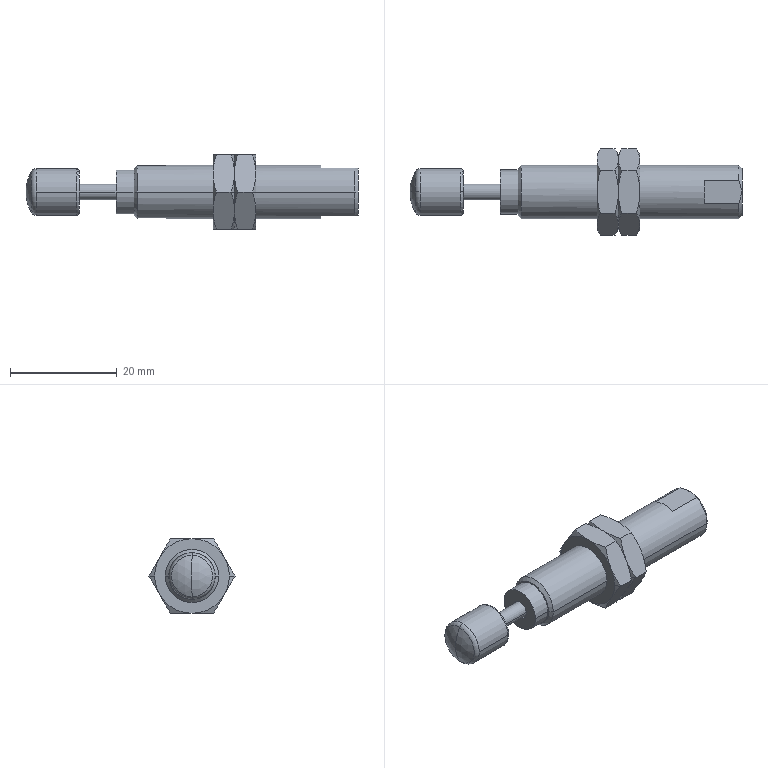Part | STEP file | RJ1007LU_0_^Buffer motion shaft | 3 solids | 89 faces | box 62.3 x 16.166 x 14 mm | volume 4876 mm3 | cone 44 | plane 25 | cylinder 14 | torus 4 | sphere 2 | commonest cylinder face diameters 8.917 x4 3 x2 3.5 x2 8.3 x2 8.7 x2 10 x2